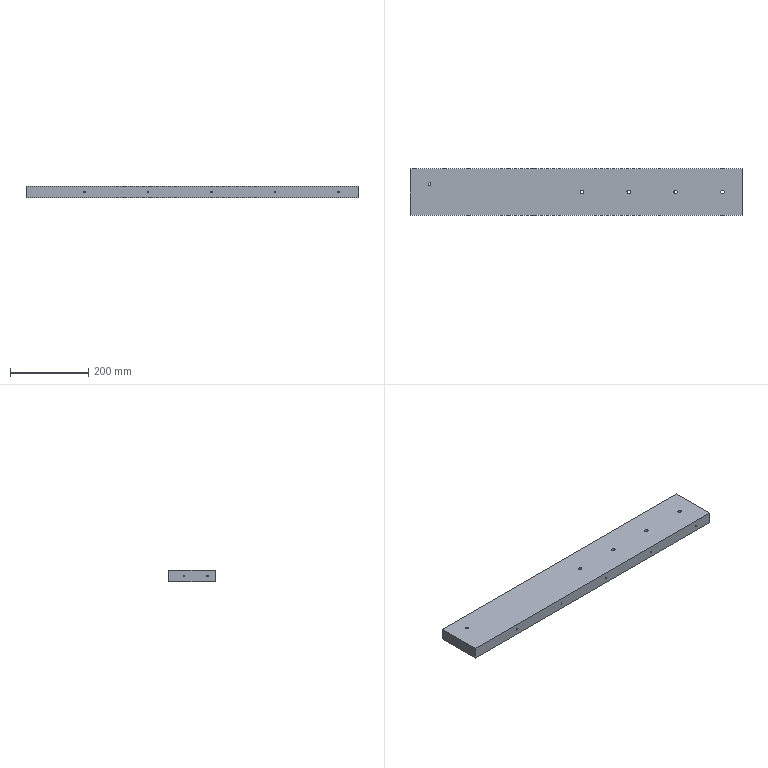Part | NX | 1 solid | 43 faces | box 850 x 120 x 30 mm | volume 3045845 mm3 | cylinder 21 | cone 16 | plane 6 | commonest cylinder face diameters 3.3 x12 9 x4 6.8 x3 8.5 x2
STEP:
#1=CARTESIAN_POINT('',(-425.,-60.,-15.));
#2=VERTEX_POINT('',#1);
#3=CARTESIAN_POINT('',(425.,-60.,-15.));
#4=VERTEX_POINT('',#3);
#5=CARTESIAN_POINT('',(-425.,-60.,-15.));
#6=DIRECTION('',(1.,0.,0.));
#7=VECTOR('',#6,1000.);
#8=LINE('',#5,#7);
#9=EDGE_CURVE('',#2,#4,#8,.T.);
#10=ORIENTED_EDGE('',*,*,#9,.T.);
#11=CARTESIAN_POINT('',(425.,-60.,15.));
#12=VERTEX_POINT('',#11);
#13=CARTESIAN_POINT('',(425.,-60.,15.));
#14=DIRECTION('',(0.,0.,-1.));
#15=VECTOR('',#14,1000.);
#16=LINE('',#13,#15);
#17=EDGE_CURVE('',#12,#4,#16,.T.);
#18=ORIENTED_EDGE('',*,*,#17,.F.);
#19=CARTESIAN_POINT('',(-425.,-60.,15.));
#20=VERTEX_POINT('',#19);
#21=CARTESIAN_POINT('',(-425.,-60.,15.));
#22=DIRECTION('',(1.,0.,0.));
#23=VECTOR('',#22,1000.);
#24=LINE('',#21,#23);
#25=EDGE_CURVE('',#20,#12,#24,.T.);
#26=ORIENTED_EDGE('',*,*,#25,.F.);
#27=CARTESIAN_POINT('',(-425.,-60.,15.));
#28=DIRECTION('',(0.,0.,-1.));
#29=VECTOR('',#28,1000.);
#30=LINE('',#27,#29);
#31=EDGE_CURVE('',#20,#2,#30,.T.);
#32=ORIENTED_EDGE('',*,*,#31,.T.);
#33=EDGE_LOOP('',(#10,#18,#26,#32));
#34=FACE_BOUND('',#33,.T.);
#35=CARTESIAN_POINT('',(375.,-60.,-1.65));
#36=VERTEX_POINT('',#35);
#37=CARTESIAN_POINT('',(375.,-60.,0.));
#38=DIRECTION('',(0.,-1.,0.));
#39=DIRECTION('',(0.,0.,-1.));
#40=AXIS2_PLACEMENT_3D('',#37,#38,#39);
#41=CIRCLE('',#40,1.65);
#42=EDGE_CURVE('',#36,#36,#41,.T.);
#43=ORIENTED_EDGE('',*,*,#42,.F.);
#44=EDGE_LOOP('',(#43));
#45=FACE_BOUND('',#44,.T.);
#46=CARTESIAN_POINT('',(212.5,-60.,-1.65));
#47=VERTEX_POINT('',#46);
#48=CARTESIAN_POINT('',(212.5,-60.,0.));
#49=DIRECTION('',(0.,-1.,0.));
#50=DIRECTION('',(0.,0.,-1.));
#51=AXIS2_PLACEMENT_3D('',#48,#49,#50);
#52=CIRCLE('',#51,1.65);
#53=EDGE_CURVE('',#47,#47,#52,.T.);
#54=ORIENTED_EDGE('',*,*,#53,.F.);
#55=EDGE_LOOP('',(#54));
#56=FACE_BOUND('',#55,.T.);
#57=CARTESIAN_POINT('',(50.,-60.,-1.65));
#58=VERTEX_POINT('',#57);
#59=CARTESIAN_POINT('',(50.,-60.,0.));
#60=DIRECTION('',(0.,-1.,0.));
#61=DIRECTION('',(0.,0.,-1.));
#62=AXIS2_PLACEMENT_3D('',#59,#60,#61);
#63=CIRCLE('',#62,1.65);
#64=EDGE_CURVE('',#58,#58,#63,.T.);
#65=ORIENTED_EDGE('',*,*,#64,.F.);
#66=EDGE_LOOP('',(#65));
#67=FACE_BOUND('',#66,.T.);
#68=CARTESIAN_POINT('',(-112.5,-60.,1.65));
#69=VERTEX_POINT('',#68);
#70=CARTESIAN_POINT('',(-112.5,-60.,0.));
#71=DIRECTION('',(0.,-1.,0.));
#72=DIRECTION('',(0.,0.,1.));
#73=AXIS2_PLACEMENT_3D('',#70,#71,#72);
#74=CIRCLE('',#73,1.65);
#75=EDGE_CURVE('',#69,#69,#74,.T.);
#76=ORIENTED_EDGE('',*,*,#75,.F.);
#77=EDGE_LOOP('',(#76));
#78=FACE_BOUND('',#77,.T.);
#79=CARTESIAN_POINT('',(-275.,-60.,1.65));
#80=VERTEX_POINT('',#79);
#81=CARTESIAN_POINT('',(-275.,-60.,0.));
#82=DIRECTION('',(0.,-1.,0.));
#83=DIRECTION('',(0.,0.,1.));
#84=AXIS2_PLACEMENT_3D('',#81,#82,#83);
#85=CIRCLE('',#84,1.65);
#86=EDGE_CURVE('',#80,#80,#85,.T.);
#87=ORIENTED_EDGE('',*,*,#86,.F.);
#88=EDGE_LOOP('',(#87));
#89=FACE_BOUND('',#88,.T.);
#90=CARTESIAN_POINT('',(-425.,-60.,15.));
#91=DIRECTION('',(0.,1.,0.));
#92=DIRECTION('',(0.,0.,1.));
#93=AXIS2_PLACEMENT_3D('',#90,#91,#92);
#94=PLANE('',#93);
#95=ADVANCED_FACE('',(#34,#45,#56,#67,#78,#89),#94,.F.);
#96=CARTESIAN_POINT('',(-425.,60.,-15.));
#97=VERTEX_POINT('',#96);
#98=CARTESIAN_POINT('',(-425.,-60.,-15.));
#99=DIRECTION('',(0.,1.,0.));
#100=VECTOR('',#99,1000.);
#101=LINE('',#98,#100);
#102=EDGE_CURVE('',#2,#97,#101,.T.);
#103=ORIENTED_EDGE('',*,*,#102,.F.);
#104=ORIENTED_EDGE('',*,*,#31,.F.);
#105=CARTESIAN_POINT('',(-425.,60.,15.));
#106=VERTEX_POINT('',#105);
#107=CARTESIAN_POINT('',(-425.,-60.,15.));
#108=DIRECTION('',(0.,1.,0.));
#109=VECTOR('',#108,1000.);
#110=LINE('',#107,#109);
#111=EDGE_CURVE('',#20,#106,#110,.T.);
#112=ORIENTED_EDGE('',*,*,#111,.T.);
#113=CARTESIAN_POINT('',(-425.,60.,15.));
#114=DIRECTION('',(0.,0.,-1.));
#115=VECTOR('',#114,1000.);
#116=LINE('',#113,#115);
#117=EDGE_CURVE('',#106,#97,#116,.T.);
#118=ORIENTED_EDGE('',*,*,#117,.T.);
#119=EDGE_LOOP('',(#103,#104,#112,#118));
#120=FACE_BOUND('',#119,.T.);
#121=CARTESIAN_POINT('',(-425.,20.,1.65));
#122=VERTEX_POINT('',#121);
#123=CARTESIAN_POINT('',(-425.,20.,0.));
#124=DIRECTION('',(-1.,0.,0.));
#125=DIRECTION('',(0.,0.,1.));
#126=AXIS2_PLACEMENT_3D('',#123,#124,#125);
#127=CIRCLE('',#126,1.65);
#128=EDGE_CURVE('',#122,#122,#127,.T.);
#129=ORIENTED_EDGE('',*,*,#128,.F.);
#130=EDGE_LOOP('',(#129));
#131=FACE_BOUND('',#130,.T.);
#132=CARTESIAN_POINT('',(-425.,-40.,1.65));
#133=VERTEX_POINT('',#132);
#134=CARTESIAN_POINT('',(-425.,-40.,0.));
#135=DIRECTION('',(-1.,0.,0.));
#136=DIRECTION('',(0.,0.,1.));
#137=AXIS2_PLACEMENT_3D('',#134,#135,#136);
#138=CIRCLE('',#137,1.65);
#139=EDGE_CURVE('',#133,#133,#138,.T.);
#140=ORIENTED_EDGE('',*,*,#139,.F.);
#141=EDGE_LOOP('',(#140));
#142=FACE_BOUND('',#141,.T.);
#143=CARTESIAN_POINT('',(-425.,-60.,15.));
#144=DIRECTION('',(-1.,0.,0.));
#145=DIRECTION('',(0.,0.,1.));
#146=AXIS2_PLACEMENT_3D('',#143,#144,#145);
#147=PLANE('',#146);
#148=ADVANCED_FACE('',(#120,#131,#142),#147,.T.);
#149=CARTESIAN_POINT('',(-335.,60.,3.4));
#150=VERTEX_POINT('',#149);
#151=CARTESIAN_POINT('',(-335.,60.,0.));
#152=DIRECTION('',(0.,1.,0.));
#153=DIRECTION('',(0.,0.,1.));
#154=AXIS2_PLACEMENT_3D('',#151,#152,#153);
#155=CIRCLE('',#154,3.4);
#156=EDGE_CURVE('',#150,#150,#155,.T.);
#157=ORIENTED_EDGE('',*,*,#156,.F.);
#158=EDGE_LOOP('',(#157));
#159=FACE_BOUND('',#158,.T.);
#160=CARTESIAN_POINT('',(425.,60.,15.));
#161=VERTEX_POINT('',#160);
#162=CARTESIAN_POINT('',(425.,60.,-15.));
#163=VERTEX_POINT('',#162);
#164=CARTESIAN_POINT('',(425.,60.,15.));
#165=DIRECTION('',(0.,0.,-1.));
#166=VECTOR('',#165,1000.);
#167=LINE('',#164,#166);
#168=EDGE_CURVE('',#161,#163,#167,.T.);
#169=ORIENTED_EDGE('',*,*,#168,.T.);
#170=CARTESIAN_POINT('',(-425.,60.,-15.));
#171=DIRECTION('',(1.,0.,0.));
#172=VECTOR('',#171,1000.);
#173=LINE('',#170,#172);
#174=EDGE_CURVE('',#163,#97,#173,.F.);
#175=ORIENTED_EDGE('',*,*,#174,.T.);
#176=ORIENTED_EDGE('',*,*,#117,.F.);
#177=CARTESIAN_POINT('',(-425.,60.,15.));
#178=DIRECTION('',(1.,0.,0.));
#179=VECTOR('',#178,1000.);
#180=LINE('',#177,#179);
#181=EDGE_CURVE('',#106,#161,#180,.T.);
#182=ORIENTED_EDGE('',*,*,#181,.T.);
#183=EDGE_LOOP('',(#169,#175,#176,#182));
#184=FACE_BOUND('',#183,.T.);
#185=CARTESIAN_POINT('',(-275.,60.,1.65));
#186=VERTEX_POINT('',#185);
#187=CARTESIAN_POINT('',(-275.,60.,0.));
#188=DIRECTION('',(0.,1.,0.));
#189=DIRECTION('',(0.,0.,1.));
#190=AXIS2_PLACEMENT_3D('',#187,#188,#189);
#191=CIRCLE('',#190,1.65);
#192=EDGE_CURVE('',#186,#186,#191,.T.);
#193=ORIENTED_EDGE('',*,*,#192,.F.);
#194=EDGE_LOOP('',(#193));
#195=FACE_BOUND('',#194,.T.);
#196=CARTESIAN_POINT('',(-112.5,60.,1.65));
#197=VERTEX_POINT('',#196);
#198=CARTESIAN_POINT('',(-112.5,60.,0.));
#199=DIRECTION('',(0.,1.,0.));
#200=DIRECTION('',(0.,0.,1.));
#201=AXIS2_PLACEMENT_3D('',#198,#199,#200);
#202=CIRCLE('',#201,1.65);
#203=EDGE_CURVE('',#197,#197,#202,.T.);
#204=ORIENTED_EDGE('',*,*,#203,.F.);
#205=EDGE_LOOP('',(#204));
#206=FACE_BOUND('',#205,.T.);
#207=CARTESIAN_POINT('',(50.,60.,1.65));
#208=VERTEX_POINT('',#207);
#209=CARTESIAN_POINT('',(50.,60.,0.));
#210=DIRECTION('',(0.,1.,0.));
#211=DIRECTION('',(0.,0.,1.));
#212=AXIS2_PLACEMENT_3D('',#209,#210,#211);
#213=CIRCLE('',#212,1.65);
#214=EDGE_CURVE('',#208,#208,#213,.T.);
#215=ORIENTED_EDGE('',*,*,#214,.F.);
#216=EDGE_LOOP('',(#215));
#217=FACE_BOUND('',#216,.T.);
#218=CARTESIAN_POINT('',(212.5,60.,1.65));
#219=VERTEX_POINT('',#218);
#220=CARTESIAN_POINT('',(212.5,60.,0.));
#221=DIRECTION('',(0.,1.,0.));
#222=DIRECTION('',(0.,0.,1.));
#223=AXIS2_PLACEMENT_3D('',#220,#221,#222);
#224=CIRCLE('',#223,1.65);
#225=EDGE_CURVE('',#219,#219,#224,.T.);
#226=ORIENTED_EDGE('',*,*,#225,.F.);
#227=EDGE_LOOP('',(#226));
#228=FACE_BOUND('',#227,.T.);
#229=CARTESIAN_POINT('',(375.,60.,1.65));
#230=VERTEX_POINT('',#229);
#231=CARTESIAN_POINT('',(375.,60.,0.));
#232=DIRECTION('',(0.,1.,0.));
#233=DIRECTION('',(0.,0.,1.));
#234=AXIS2_PLACEMENT_3D('',#231,#232,#233);
#235=CIRCLE('',#234,1.65);
#236=EDGE_CURVE('',#230,#230,#235,.T.);
#237=ORIENTED_EDGE('',*,*,#236,.F.);
#238=EDGE_LOOP('',(#237));
#239=FACE_BOUND('',#238,.T.);
#240=CARTESIAN_POINT('',(-415.,60.,3.4));
#241=VERTEX_POINT('',#240);
#242=CARTESIAN_POINT('',(-415.,60.,0.));
#243=DIRECTION('',(0.,1.,0.));
#244=DIRECTION('',(0.,0.,1.));
#245=AXIS2_PLACEMENT_3D('',#242,#243,#244);
#246=CIRCLE('',#245,3.4);
#247=EDGE_CURVE('',#241,#241,#246,.T.);
#248=ORIENTED_EDGE('',*,*,#247,.F.);
#249=EDGE_LOOP('',(#248));
#250=FACE_BOUND('',#249,.T.);
#251=CARTESIAN_POINT('',(-425.,60.,15.));
#252=DIRECTION('',(0.,1.,0.));
#253=DIRECTION('',(0.,0.,1.));
#254=AXIS2_PLACEMENT_3D('',#251,#252,#253);
#255=PLANE('',#254);
#256=ADVANCED_FACE('',(#159,#184,#195,#206,#217,#228,#239,#250),#255,.T.);
#257=ORIENTED_EDGE('',*,*,#168,.F.);
#258=CARTESIAN_POINT('',(425.,-60.,15.));
#259=DIRECTION('',(0.,-1.,0.));
#260=VECTOR('',#259,1000.);
#261=LINE('',#258,#260);
#262=EDGE_CURVE('',#161,#12,#261,.T.);
#263=ORIENTED_EDGE('',*,*,#262,.T.);
#264=ORIENTED_EDGE('',*,*,#17,.T.);
#265=CARTESIAN_POINT('',(425.,0.,-15.));
#266=DIRECTION('',(0.,1.,0.));
#267=VECTOR('',#266,1000.);
#268=LINE('',#265,#267);
#269=EDGE_CURVE('',#4,#163,#268,.T.);
#270=ORIENTED_EDGE('',*,*,#269,.T.);
#271=EDGE_LOOP('',(#257,#263,#264,#270));
#272=FACE_BOUND('',#271,.T.);
#273=CARTESIAN_POINT('',(425.,45.,-4.25));
#274=VERTEX_POINT('',#273);
#275=CARTESIAN_POINT('',(425.,45.,0.));
#276=DIRECTION('',(1.,0.,0.));
#277=DIRECTION('',(0.,0.,-1.));
#278=AXIS2_PLACEMENT_3D('',#275,#276,#277);
#279=CIRCLE('',#278,4.25);
#280=EDGE_CURVE('',#274,#274,#279,.T.);
#281=ORIENTED_EDGE('',*,*,#280,.F.);
#282=EDGE_LOOP('',(#281));
#283=FACE_BOUND('',#282,.T.);
#284=CARTESIAN_POINT('',(425.,-45.,-4.25));
#285=VERTEX_POINT('',#284);
#286=CARTESIAN_POINT('',(425.,-45.,0.));
#287=DIRECTION('',(1.,0.,0.));
#288=DIRECTION('',(0.,0.,-1.));
#289=AXIS2_PLACEMENT_3D('',#286,#287,#288);
#290=CIRCLE('',#289,4.25);
#291=EDGE_CURVE('',#285,#285,#290,.T.);
#292=ORIENTED_EDGE('',*,*,#291,.F.);
#293=EDGE_LOOP('',(#292));
#294=FACE_BOUND('',#293,.T.);
#295=CARTESIAN_POINT('',(425.,-60.,15.));
#296=DIRECTION('',(-1.,0.,0.));
#297=DIRECTION('',(0.,0.,1.));
#298=AXIS2_PLACEMENT_3D('',#295,#296,#297);
#299=PLANE('',#298);
#300=ADVANCED_FACE('',(#272,#283,#294),#299,.F.);
#301=CARTESIAN_POINT('',(139.5,0.,-15.));
#302=VERTEX_POINT('',#301);
#303=CARTESIAN_POINT('',(135.,0.,-15.));
#304=DIRECTION('',(0.,0.,1.));
#305=DIRECTION('',(1.,0.,0.));
#306=AXIS2_PLACEMENT_3D('',#303,#304,#305);
#307=CIRCLE('',#306,4.5);
#308=EDGE_CURVE('',#302,#302,#307,.T.);
#309=ORIENTED_EDGE('',*,*,#308,.T.);
#310=EDGE_LOOP('',(#309));
#311=FACE_BOUND('',#310,.T.);
#312=CARTESIAN_POINT('',(19.5,0.,-15.));
#313=VERTEX_POINT('',#312);
#314=CARTESIAN_POINT('',(15.,0.,-15.));
#315=DIRECTION('',(0.,0.,1.));
#316=DIRECTION('',(1.,0.,0.));
#317=AXIS2_PLACEMENT_3D('',#314,#315,#316);
#318=CIRCLE('',#317,4.5);
#319=EDGE_CURVE('',#313,#313,#318,.T.);
#320=ORIENTED_EDGE('',*,*,#319,.T.);
#321=EDGE_LOOP('',(#320));
#322=FACE_BOUND('',#321,.T.);
#323=ORIENTED_EDGE('',*,*,#174,.F.);
#324=ORIENTED_EDGE('',*,*,#269,.F.);
#325=ORIENTED_EDGE('',*,*,#9,.F.);
#326=ORIENTED_EDGE('',*,*,#102,.T.);
#327=EDGE_LOOP('',(#323,#324,#325,#326));
#328=FACE_BOUND('',#327,.T.);
#329=CARTESIAN_POINT('',(259.5,0.,-15.));
#330=VERTEX_POINT('',#329);
#331=CARTESIAN_POINT('',(255.,0.,-15.));
#332=DIRECTION('',(0.,0.,1.));
#333=DIRECTION('',(1.,0.,0.));
#334=AXIS2_PLACEMENT_3D('',#331,#332,#333);
#335=CIRCLE('',#334,4.5);
#336=EDGE_CURVE('',#330,#330,#335,.T.);
#337=ORIENTED_EDGE('',*,*,#336,.T.);
#338=EDGE_LOOP('',(#337));
#339=FACE_BOUND('',#338,.T.);
#340=CARTESIAN_POINT('',(379.5,0.,-15.));
#341=VERTEX_POINT('',#340);
#342=CARTESIAN_POINT('',(375.,0.,-15.));
#343=DIRECTION('',(0.,0.,1.));
#344=DIRECTION('',(1.,0.,0.));
#345=AXIS2_PLACEMENT_3D('',#342,#343,#344);
#346=CIRCLE('',#345,4.5);
#347=EDGE_CURVE('',#341,#341,#346,.T.);
#348=ORIENTED_EDGE('',*,*,#347,.T.);
#349=EDGE_LOOP('',(#348));
#350=FACE_BOUND('',#349,.T.);
#351=CARTESIAN_POINT('',(-378.4,20.,-15.));
#352=VERTEX_POINT('',#351);
#353=CARTESIAN_POINT('',(-375.,20.,-15.));
#354=DIRECTION('',(0.,0.,-1.));
#355=DIRECTION('',(-1.,0.,0.));
#356=AXIS2_PLACEMENT_3D('',#353,#354,#355);
#357=CIRCLE('',#356,3.4);
#358=EDGE_CURVE('',#352,#352,#357,.T.);
#359=ORIENTED_EDGE('',*,*,#358,.F.);
#360=EDGE_LOOP('',(#359));
#361=FACE_BOUND('',#360,.T.);
#362=CARTESIAN_POINT('',(0.,0.,-15.));
#363=DIRECTION('',(0.,0.,-1.));
#364=DIRECTION('',(-1.,0.,0.));
#365=AXIS2_PLACEMENT_3D('',#362,#363,#364);
#366=PLANE('',#365);
#367=ADVANCED_FACE('',(#311,#322,#328,#339,#350,#361),#366,.T.);
#368=CARTESIAN_POINT('',(259.5,0.,15.));
#369=VERTEX_POINT('',#368);
#370=CARTESIAN_POINT('',(255.,0.,15.));
#371=DIRECTION('',(0.,0.,1.));
#372=DIRECTION('',(1.,0.,0.));
#373=AXIS2_PLACEMENT_3D('',#370,#371,#372);
#374=CIRCLE('',#373,4.5);
#375=EDGE_CURVE('',#369,#369,#374,.T.);
#376=ORIENTED_EDGE('',*,*,#375,.F.);
#377=EDGE_LOOP('',(#376));
#378=FACE_BOUND('',#377,.T.);
#379=ORIENTED_EDGE('',*,*,#262,.F.);
#380=ORIENTED_EDGE('',*,*,#181,.F.);
#381=ORIENTED_EDGE('',*,*,#111,.F.);
#382=ORIENTED_EDGE('',*,*,#25,.T.);
#383=EDGE_LOOP('',(#379,#380,#381,#382));
#384=FACE_BOUND('',#383,.T.);
#385=CARTESIAN_POINT('',(19.5,0.,15.));
#386=VERTEX_POINT('',#385);
#387=CARTESIAN_POINT('',(15.,0.,15.));
#388=DIRECTION('',(0.,0.,1.));
#389=DIRECTION('',(1.,0.,0.));
#390=AXIS2_PLACEMENT_3D('',#387,#388,#389);
#391=CIRCLE('',#390,4.5);
#392=EDGE_CURVE('',#386,#386,#391,.T.);
#393=ORIENTED_EDGE('',*,*,#392,.F.);
#394=EDGE_LOOP('',(#393));
#395=FACE_BOUND('',#394,.T.);
#396=CARTESIAN_POINT('',(139.5,0.,15.));
#397=VERTEX_POINT('',#396);
#398=CARTESIAN_POINT('',(135.,0.,15.));
#399=DIRECTION('',(0.,0.,1.));
#400=DIRECTION('',(1.,0.,0.));
#401=AXIS2_PLACEMENT_3D('',#398,#399,#400);
#402=CIRCLE('',#401,4.5);
#403=EDGE_CURVE('',#397,#397,#402,.T.);
#404=ORIENTED_EDGE('',*,*,#403,.F.);
#405=EDGE_LOOP('',(#404));
#406=FACE_BOUND('',#405,.T.);
#407=CARTESIAN_POINT('',(379.5,0.,15.));
#408=VERTEX_POINT('',#407);
#409=CARTESIAN_POINT('',(375.,0.,15.));
#410=DIRECTION('',(0.,0.,1.));
#411=DIRECTION('',(1.,0.,0.));
#412=AXIS2_PLACEMENT_3D('',#409,#410,#411);
#413=CIRCLE('',#412,4.5);
#414=EDGE_CURVE('',#408,#408,#413,.T.);
#415=ORIENTED_EDGE('',*,*,#414,.F.);
#416=EDGE_LOOP('',(#415));
#417=FACE_BOUND('',#416,.T.);
#418=CARTESIAN_POINT('',(-378.4,20.,15.));
#419=VERTEX_POINT('',#418);
#420=CARTESIAN_POINT('',(-375.,20.,15.));
#421=DIRECTION('',(0.,0.,-1.));
#422=DIRECTION('',(-1.,0.,0.));
#423=AXIS2_PLACEMENT_3D('',#420,#421,#422);
#424=CIRCLE('',#423,3.4);
#425=EDGE_CURVE('',#419,#419,#424,.T.);
#426=ORIENTED_EDGE('',*,*,#425,.T.);
#427=EDGE_LOOP('',(#426));
#428=FACE_BOUND('',#427,.T.);
#429=CARTESIAN_POINT('',(0.,0.,15.));
#430=DIRECTION('',(0.,0.,-1.));
#431=DIRECTION('',(-1.,0.,0.));
#432=AXIS2_PLACEMENT_3D('',#429,#430,#431);
#433=PLANE('',#432);
#434=ADVANCED_FACE('',(#378,#384,#395,#406,#417,#428),#433,.F.);
#435=CARTESIAN_POINT('',(-335.,40.25,3.4));
#436=VERTEX_POINT('',#435);
#437=CARTESIAN_POINT('',(-335.,40.25,0.));
#438=DIRECTION('',(0.,1.,0.));
#439=DIRECTION('',(0.,0.,1.));
#440=AXIS2_PLACEMENT_3D('',#437,#438,#439);
#441=CIRCLE('',#440,3.4);
#442=EDGE_CURVE('',#436,#436,#441,.T.);
#443=ORIENTED_EDGE('',*,*,#442,.T.);
#444=EDGE_LOOP('',(#443));
#445=FACE_BOUND('',#444,.T.);
#446=CARTESIAN_POINT('',(-335.,38.207,0.));
#447=VERTEX_POINT('',#446);
#448=VERTEX_LOOP('',#447);
#449=FACE_BOUND('',#448,.T.);
#450=CARTESIAN_POINT('',(-335.,40.25,0.));
#451=DIRECTION('',(0.,1.,0.));
#452=DIRECTION('',(0.,0.,1.));
#453=AXIS2_PLACEMENT_3D('',#450,#451,#452);
#454=CONICAL_SURFACE('',#453,3.4,1.03);
#455=ADVANCED_FACE('',(#445,#449),#454,.F.);
#456=ORIENTED_EDGE('',*,*,#442,.F.);
#457=EDGE_LOOP('',(#456));
#458=FACE_BOUND('',#457,.T.);
#459=ORIENTED_EDGE('',*,*,#156,.T.);
#460=EDGE_LOOP('',(#459));
#461=FACE_BOUND('',#460,.T.);
#462=CARTESIAN_POINT('',(-335.,60.,0.));
#463=DIRECTION('',(0.,1.,0.));
#464=DIRECTION('',(0.,0.,1.));
#465=AXIS2_PLACEMENT_3D('',#462,#463,#464);
#466=CYLINDRICAL_SURFACE('',#465,3.4);
#467=ADVANCED_FACE('',(#458,#461),#466,.F.);
#468=CARTESIAN_POINT('',(-415.,40.25,3.4));
#469=VERTEX_POINT('',#468);
#470=CARTESIAN_POINT('',(-415.,40.25,0.));
#471=DIRECTION('',(0.,1.,0.));
#472=DIRECTION('',(0.,0.,1.));
#473=AXIS2_PLACEMENT_3D('',#470,#471,#472);
#474=CIRCLE('',#473,3.4);
#475=EDGE_CURVE('',#469,#469,#474,.T.);
#476=ORIENTED_EDGE('',*,*,#475,.T.);
#477=EDGE_LOOP('',(#476));
#478=FACE_BOUND('',#477,.T.);
#479=CARTESIAN_POINT('',(-415.,38.207,0.));
#480=VERTEX_POINT('',#479);
#481=VERTEX_LOOP('',#480);
#482=FACE_BOUND('',#481,.T.);
#483=CARTESIAN_POINT('',(-415.,40.25,0.));
#484=DIRECTION('',(0.,1.,0.));
#485=DIRECTION('',(0.,0.,1.));
#486=AXIS2_PLACEMENT_3D('',#483,#484,#485);
#487=CONICAL_SURFACE('',#486,3.4,1.03);
#488=ADVANCED_FACE('',(#478,#482),#487,.F.);
#489=ORIENTED_EDGE('',*,*,#475,.F.);
#490=EDGE_LOOP('',(#489));
#491=FACE_BOUND('',#490,.T.);
#492=ORIENTED_EDGE('',*,*,#247,.T.);
#493=EDGE_LOOP('',(#492));
#494=FACE_BOUND('',#493,.T.);
#495=CARTESIAN_POINT('',(-415.,60.,0.));
#496=DIRECTION('',(0.,1.,0.));
#497=DIRECTION('',(0.,0.,1.));
#498=AXIS2_PLACEMENT_3D('',#495,#496,#497);
#499=CYLINDRICAL_SURFACE('',#498,3.4);
#500=ADVANCED_FACE('',(#491,#494),#499,.F.);
#501=CARTESIAN_POINT('',(397.946,45.,0.));
#502=VERTEX_POINT('',#501);
#503=VERTEX_LOOP('',#502);
#504=FACE_BOUND('',#503,.T.);
#505=CARTESIAN_POINT('',(400.5,45.,-4.25));
#506=VERTEX_POINT('',#505);
#507=CARTESIAN_POINT('',(400.5,45.,0.));
#508=DIRECTION('',(1.,0.,0.));
#509=DIRECTION('',(0.,0.,-1.));
#510=AXIS2_PLACEMENT_3D('',#507,#508,#509);
#511=CIRCLE('',#510,4.25);
#512=EDGE_CURVE('',#506,#506,#511,.T.);
#513=ORIENTED_EDGE('',*,*,#512,.T.);
#514=EDGE_LOOP('',(#513));
#515=FACE_BOUND('',#514,.T.);
#516=CARTESIAN_POINT('',(400.5,45.,0.));
#517=DIRECTION('',(1.,0.,0.));
#518=DIRECTION('',(0.,0.,-1.));
#519=AXIS2_PLACEMENT_3D('',#516,#517,#518);
#520=CONICAL_SURFACE('',#519,4.25,1.03);
#521=ADVANCED_FACE('',(#504,#515),#520,.F.);
#522=ORIENTED_EDGE('',*,*,#280,.T.);
#523=EDGE_LOOP('',(#522));
#524=FACE_BOUND('',#523,.T.);
#525=ORIENTED_EDGE('',*,*,#512,.F.);
#526=EDGE_LOOP('',(#525));
#527=FACE_BOUND('',#526,.T.);
#528=CARTESIAN_POINT('',(425.,45.,0.));
#529=DIRECTION('',(1.,0.,0.));
#530=DIRECTION('',(0.,0.,-1.));
#531=AXIS2_PLACEMENT_3D('',#528,#529,#530);
#532=CYLINDRICAL_SURFACE('',#531,4.25);
#533=ADVANCED_FACE('',(#524,#527),#532,.F.);
#534=CARTESIAN_POINT('',(397.946,-45.,0.));
#535=VERTEX_POINT('',#534);
#536=VERTEX_LOOP('',#535);
#537=FACE_BOUND('',#536,.T.);
#538=CARTESIAN_POINT('',(400.5,-45.,-4.25));
#539=VERTEX_POINT('',#538);
#540=CARTESIAN_POINT('',(400.5,-45.,0.));
#541=DIRECTION('',(1.,0.,0.));
#542=DIRECTION('',(0.,0.,-1.));
#543=AXIS2_PLACEMENT_3D('',#540,#541,#542);
#544=CIRCLE('',#543,4.25);
#545=EDGE_CURVE('',#539,#539,#544,.T.);
#546=ORIENTED_EDGE('',*,*,#545,.T.);
#547=EDGE_LOOP('',(#546));
#548=FACE_BOUND('',#547,.T.);
#549=CARTESIAN_POINT('',(400.5,-45.,0.));
#550=DIRECTION('',(1.,0.,0.));
#551=DIRECTION('',(0.,0.,-1.));
#552=AXIS2_PLACEMENT_3D('',#549,#550,#551);
#553=CONICAL_SURFACE('',#552,4.25,1.03);
#554=ADVANCED_FACE('',(#537,#548),#553,.F.);
#555=ORIENTED_EDGE('',*,*,#291,.T.);
#556=EDGE_LOOP('',(#555));
#557=FACE_BOUND('',#556,.T.);
#558=ORIENTED_EDGE('',*,*,#545,.F.);
#559=EDGE_LOOP('',(#558));
#560=FACE_BOUND('',#559,.T.);
#561=CARTESIAN_POINT('',(425.,-45.,0.));
#562=DIRECTION('',(1.,0.,0.));
#563=DIRECTION('',(0.,0.,-1.));
#564=AXIS2_PLACEMENT_3D('',#561,#562,#563);
#565=CYLINDRICAL_SURFACE('',#564,4.25);
#566=ADVANCED_FACE('',(#557,#560),#565,.F.);
#567=ORIENTED_EDGE('',*,*,#319,.F.);
#568=EDGE_LOOP('',(#567));
#569=FACE_BOUND('',#568,.T.);
#570=ORIENTED_EDGE('',*,*,#392,.T.);
#571=EDGE_LOOP('',(#570));
#572=FACE_BOUND('',#571,.T.);
#573=CARTESIAN_POINT('',(15.,0.,15.));
#574=DIRECTION('',(0.,0.,1.));
#575=DIRECTION('',(1.,0.,0.));
#576=AXIS2_PLACEMENT_3D('',#573,#574,#575);
#577=CYLINDRICAL_SURFACE('',#576,4.5);
#578=ADVANCED_FACE('',(#569,#572),#577,.F.);
#579=ORIENTED_EDGE('',*,*,#308,.F.);
#580=EDGE_LOOP('',(#579));
#581=FACE_BOUND('',#580,.T.);
#582=ORIENTED_EDGE('',*,*,#403,.T.);
#583=EDGE_LOOP('',(#582));
#584=FACE_BOUND('',#583,.T.);
#585=CARTESIAN_POINT('',(135.,0.,15.));
#586=DIRECTION('',(0.,0.,1.));
#587=DIRECTION('',(1.,0.,0.));
#588=AXIS2_PLACEMENT_3D('',#585,#586,#587);
#589=CYLINDRICAL_SURFACE('',#588,4.5);
#590=ADVANCED_FACE('',(#581,#584),#589,.F.);
#591=ORIENTED_EDGE('',*,*,#336,.F.);
#592=EDGE_LOOP('',(#591));
#593=FACE_BOUND('',#592,.T.);
#594=ORIENTED_EDGE('',*,*,#375,.T.);
#595=EDGE_LOOP('',(#594));
#596=FACE_BOUND('',#595,.T.);
#597=CARTESIAN_POINT('',(255.,0.,15.));
#598=DIRECTION('',(0.,0.,1.));
#599=DIRECTION('',(1.,0.,0.));
#600=AXIS2_PLACEMENT_3D('',#597,#598,#599);
#601=CYLINDRICAL_SURFACE('',#600,4.5);
#602=ADVANCED_FACE('',(#593,#596),#601,.F.);
#603=ORIENTED_EDGE('',*,*,#347,.F.);
#604=EDGE_LOOP('',(#603));
#605=FACE_BOUND('',#604,.T.);
#606=ORIENTED_EDGE('',*,*,#414,.T.);
#607=EDGE_LOOP('',(#606));
#608=FACE_BOUND('',#607,.T.);
#609=CARTESIAN_POINT('',(375.,0.,15.));
#610=DIRECTION('',(0.,0.,1.));
#611=DIRECTION('',(1.,0.,0.));
#612=AXIS2_PLACEMENT_3D('',#609,#610,#611);
#613=CYLINDRICAL_SURFACE('',#612,4.5);
#614=ADVANCED_FACE('',(#605,#608),#613,.F.);
#615=ORIENTED_EDGE('',*,*,#358,.T.);
#616=EDGE_LOOP('',(#615));
#617=FACE_BOUND('',#616,.T.);
#618=ORIENTED_EDGE('',*,*,#425,.F.);
#619=EDGE_LOOP('',(#618));
#620=FACE_BOUND('',#619,.T.);
#621=CARTESIAN_POINT('',(-375.,20.,-15.));
#622=DIRECTION('',(0.,0.,-1.));
#623=DIRECTION('',(-1.,0.,0.));
#624=AXIS2_PLACEMENT_3D('',#621,#622,#623);
#625=CYLINDRICAL_SURFACE('',#624,3.4);
#626=ADVANCED_FACE('',(#617,#620),#625,.F.);
#627=CARTESIAN_POINT('',(-275.,49.9,1.65));
#628=VERTEX_POINT('',#627);
#629=CARTESIAN_POINT('',(-275.,49.9,0.));
#630=DIRECTION('',(0.,1.,0.));
#631=DIRECTION('',(0.,0.,1.));
#632=AXIS2_PLACEMENT_3D('',#629,#630,#631);
#633=CIRCLE('',#632,1.65);
#634=EDGE_CURVE('',#628,#628,#633,.T.);
#635=ORIENTED_EDGE('',*,*,#634,.T.);
#636=EDGE_LOOP('',(#635));
#637=FACE_BOUND('',#636,.T.);
#638=CARTESIAN_POINT('',(-275.,48.909,0.));
#639=VERTEX_POINT('',#638);
#640=VERTEX_LOOP('',#639);
#641=FACE_BOUND('',#640,.T.);
#642=CARTESIAN_POINT('',(-275.,49.9,0.));
#643=DIRECTION('',(0.,1.,0.));
#644=DIRECTION('',(0.,0.,1.));
#645=AXIS2_PLACEMENT_3D('',#642,#643,#644);
#646=CONICAL_SURFACE('',#645,1.65,1.03);
#647=ADVANCED_FACE('',(#637,#641),#646,.F.);
#648=ORIENTED_EDGE('',*,*,#634,.F.);
#649=EDGE_LOOP('',(#648));
#650=FACE_BOUND('',#649,.T.);
#651=ORIENTED_EDGE('',*,*,#192,.T.);
#652=EDGE_LOOP('',(#651));
#653=FACE_BOUND('',#652,.T.);
#654=CARTESIAN_POINT('',(-275.,60.,0.));
#655=DIRECTION('',(0.,1.,0.));
#656=DIRECTION('',(0.,0.,1.));
#657=AXIS2_PLACEMENT_3D('',#654,#655,#656);
#658=CYLINDRICAL_SURFACE('',#657,1.65);
#659=ADVANCED_FACE('',(#650,#653),#658,.F.);
#660=CARTESIAN_POINT('',(-112.5,49.9,1.65));
#661=VERTEX_POINT('',#660);
#662=CARTESIAN_POINT('',(-112.5,49.9,0.));
#663=DIRECTION('',(0.,1.,0.));
#664=DIRECTION('',(0.,0.,1.));
#665=AXIS2_PLACEMENT_3D('',#662,#663,#664);
#666=CIRCLE('',#665,1.65);
#667=EDGE_CURVE('',#661,#661,#666,.T.);
#668=ORIENTED_EDGE('',*,*,#667,.T.);
#669=EDGE_LOOP('',(#668));
#670=FACE_BOUND('',#669,.T.);
#671=CARTESIAN_POINT('',(-112.5,48.909,0.));
#672=VERTEX_POINT('',#671);
#673=VERTEX_LOOP('',#672);
#674=FACE_BOUND('',#673,.T.);
#675=CARTESIAN_POINT('',(-112.5,49.9,0.));
#676=DIRECTION('',(0.,1.,0.));
#677=DIRECTION('',(0.,0.,1.));
#678=AXIS2_PLACEMENT_3D('',#675,#676,#677);
#679=CONICAL_SURFACE('',#678,1.65,1.03);
#680=ADVANCED_FACE('',(#670,#674),#679,.F.);
#681=ORIENTED_EDGE('',*,*,#667,.F.);
#682=EDGE_LOOP('',(#681));
#683=FACE_BOUND('',#682,.T.);
#684=ORIENTED_EDGE('',*,*,#203,.T.);
#685=EDGE_LOOP('',(#684));
#686=FACE_BOUND('',#685,.T.);
#687=CARTESIAN_POINT('',(-112.5,60.,0.));
#688=DIRECTION('',(0.,1.,0.));
#689=DIRECTION('',(0.,0.,1.));
#690=AXIS2_PLACEMENT_3D('',#687,#688,#689);
#691=CYLINDRICAL_SURFACE('',#690,1.65);
#692=ADVANCED_FACE('',(#683,#686),#691,.F.);
#693=CARTESIAN_POINT('',(50.,49.9,1.65));
#694=VERTEX_POINT('',#693);
#695=CARTESIAN_POINT('',(50.,49.9,0.));
#696=DIRECTION('',(0.,1.,0.));
#697=DIRECTION('',(0.,0.,1.));
#698=AXIS2_PLACEMENT_3D('',#695,#696,#697);
#699=CIRCLE('',#698,1.65);
#700=EDGE_CURVE('',#694,#694,#699,.T.);
#701=ORIENTED_EDGE('',*,*,#700,.T.);
#702=EDGE_LOOP('',(#701));
#703=FACE_BOUND('',#702,.T.);
#704=CARTESIAN_POINT('',(50.,48.909,0.));
#705=VERTEX_POINT('',#704);
#706=VERTEX_LOOP('',#705);
#707=FACE_BOUND('',#706,.T.);
#708=CARTESIAN_POINT('',(50.,49.9,0.));
#709=DIRECTION('',(0.,1.,0.));
#710=DIRECTION('',(0.,0.,1.));
#711=AXIS2_PLACEMENT_3D('',#708,#709,#710);
#712=CONICAL_SURFACE('',#711,1.65,1.03);
#713=ADVANCED_FACE('',(#703,#707),#712,.F.);
#714=ORIENTED_EDGE('',*,*,#700,.F.);
#715=EDGE_LOOP('',(#714));
#716=FACE_BOUND('',#715,.T.);
#717=ORIENTED_EDGE('',*,*,#214,.T.);
#718=EDGE_LOOP('',(#717));
#719=FACE_BOUND('',#718,.T.);
#720=CARTESIAN_POINT('',(50.,-60.,0.));
#721=DIRECTION('',(0.,-1.,0.));
#722=DIRECTION('',(0.,0.,-1.));
#723=AXIS2_PLACEMENT_3D('',#720,#721,#722);
#724=CYLINDRICAL_SURFACE('',#723,1.65);
#725=ADVANCED_FACE('',(#716,#719),#724,.F.);
#726=CARTESIAN_POINT('',(212.5,49.9,1.65));
#727=VERTEX_POINT('',#726);
#728=CARTESIAN_POINT('',(212.5,49.9,0.));
#729=DIRECTION('',(0.,1.,0.));
#730=DIRECTION('',(0.,0.,1.));
#731=AXIS2_PLACEMENT_3D('',#728,#729,#730);
#732=CIRCLE('',#731,1.65);
#733=EDGE_CURVE('',#727,#727,#732,.T.);
#734=ORIENTED_EDGE('',*,*,#733,.T.);
#735=EDGE_LOOP('',(#734));
#736=FACE_BOUND('',#735,.T.);
#737=CARTESIAN_POINT('',(212.5,48.909,0.));
#738=VERTEX_POINT('',#737);
#739=VERTEX_LOOP('',#738);
#740=FACE_BOUND('',#739,.T.);
#741=CARTESIAN_POINT('',(212.5,49.9,0.));
#742=DIRECTION('',(0.,1.,0.));
#743=DIRECTION('',(0.,0.,1.));
#744=AXIS2_PLACEMENT_3D('',#741,#742,#743);
#745=CONICAL_SURFACE('',#744,1.65,1.03);
#746=ADVANCED_FACE('',(#736,#740),#745,.F.);
#747=ORIENTED_EDGE('',*,*,#733,.F.);
#748=EDGE_LOOP('',(#747));
#749=FACE_BOUND('',#748,.T.);
#750=ORIENTED_EDGE('',*,*,#225,.T.);
#751=EDGE_LOOP('',(#750));
#752=FACE_BOUND('',#751,.T.);
#753=CARTESIAN_POINT('',(212.5,-60.,0.));
#754=DIRECTION('',(0.,-1.,0.));
#755=DIRECTION('',(0.,0.,-1.));
#756=AXIS2_PLACEMENT_3D('',#753,#754,#755);
#757=CYLINDRICAL_SURFACE('',#756,1.65);
#758=ADVANCED_FACE('',(#749,#752),#757,.F.);
#759=CARTESIAN_POINT('',(375.,49.9,1.65));
#760=VERTEX_POINT('',#759);
#761=CARTESIAN_POINT('',(375.,49.9,0.));
#762=DIRECTION('',(0.,1.,0.));
#763=DIRECTION('',(0.,0.,1.));
#764=AXIS2_PLACEMENT_3D('',#761,#762,#763);
#765=CIRCLE('',#764,1.65);
#766=EDGE_CURVE('',#760,#760,#765,.T.);
#767=ORIENTED_EDGE('',*,*,#766,.T.);
#768=EDGE_LOOP('',(#767));
#769=FACE_BOUND('',#768,.T.);
#770=CARTESIAN_POINT('',(375.,48.909,0.));
#771=VERTEX_POINT('',#770);
#772=VERTEX_LOOP('',#771);
#773=FACE_BOUND('',#772,.T.);
#774=CARTESIAN_POINT('',(375.,49.9,0.));
#775=DIRECTION('',(0.,1.,0.));
#776=DIRECTION('',(0.,0.,1.));
#777=AXIS2_PLACEMENT_3D('',#774,#775,#776);
#778=CONICAL_SURFACE('',#777,1.65,1.03);
#779=ADVANCED_FACE('',(#769,#773),#778,.F.);
#780=ORIENTED_EDGE('',*,*,#766,.F.);
#781=EDGE_LOOP('',(#780));
#782=FACE_BOUND('',#781,.T.);
#783=ORIENTED_EDGE('',*,*,#236,.T.);
#784=EDGE_LOOP('',(#783));
#785=FACE_BOUND('',#784,.T.);
#786=CARTESIAN_POINT('',(375.,-60.,0.));
#787=DIRECTION('',(0.,-1.,0.));
#788=DIRECTION('',(0.,0.,-1.));
#789=AXIS2_PLACEMENT_3D('',#786,#787,#788);
#790=CYLINDRICAL_SURFACE('',#789,1.65);
#791=ADVANCED_FACE('',(#782,#785),#790,.F.);
#792=CARTESIAN_POINT('',(375.,-48.909,0.));
#793=VERTEX_POINT('',#792);
#794=VERTEX_LOOP('',#793);
#795=FACE_BOUND('',#794,.T.);
#796=CARTESIAN_POINT('',(375.,-49.9,-1.65));
#797=VERTEX_POINT('',#796);
#798=CARTESIAN_POINT('',(375.,-49.9,0.));
#799=DIRECTION('',(0.,-1.,0.));
#800=DIRECTION('',(0.,0.,-1.));
#801=AXIS2_PLACEMENT_3D('',#798,#799,#800);
#802=CIRCLE('',#801,1.65);
#803=EDGE_CURVE('',#797,#797,#802,.T.);
#804=ORIENTED_EDGE('',*,*,#803,.T.);
#805=EDGE_LOOP('',(#804));
#806=FACE_BOUND('',#805,.T.);
#807=CARTESIAN_POINT('',(375.,-49.9,0.));
#808=DIRECTION('',(0.,-1.,0.));
#809=DIRECTION('',(0.,0.,-1.));
#810=AXIS2_PLACEMENT_3D('',#807,#808,#809);
#811=CONICAL_SURFACE('',#810,1.65,1.03);
#812=ADVANCED_FACE('',(#795,#806),#811,.F.);
#813=ORIENTED_EDGE('',*,*,#42,.T.);
#814=EDGE_LOOP('',(#813));
#815=FACE_BOUND('',#814,.T.);
#816=ORIENTED_EDGE('',*,*,#803,.F.);
#817=EDGE_LOOP('',(#816));
#818=FACE_BOUND('',#817,.T.);
#819=CARTESIAN_POINT('',(375.,-60.,0.));
#820=DIRECTION('',(0.,-1.,0.));
#821=DIRECTION('',(0.,0.,-1.));
#822=AXIS2_PLACEMENT_3D('',#819,#820,#821);
#823=CYLINDRICAL_SURFACE('',#822,1.65);
#824=ADVANCED_FACE('',(#815,#818),#823,.F.);
#825=CARTESIAN_POINT('',(212.5,-48.909,0.));
#826=VERTEX_POINT('',#825);
#827=VERTEX_LOOP('',#826);
#828=FACE_BOUND('',#827,.T.);
#829=CARTESIAN_POINT('',(212.5,-49.9,-1.65));
#830=VERTEX_POINT('',#829);
#831=CARTESIAN_POINT('',(212.5,-49.9,0.));
#832=DIRECTION('',(0.,-1.,0.));
#833=DIRECTION('',(0.,0.,-1.));
#834=AXIS2_PLACEMENT_3D('',#831,#832,#833);
#835=CIRCLE('',#834,1.65);
#836=EDGE_CURVE('',#830,#830,#835,.T.);
#837=ORIENTED_EDGE('',*,*,#836,.T.);
#838=EDGE_LOOP('',(#837));
#839=FACE_BOUND('',#838,.T.);
#840=CARTESIAN_POINT('',(212.5,-49.9,0.));
#841=DIRECTION('',(0.,-1.,0.));
#842=DIRECTION('',(0.,0.,-1.));
#843=AXIS2_PLACEMENT_3D('',#840,#841,#842);
#844=CONICAL_SURFACE('',#843,1.65,1.03);
#845=ADVANCED_FACE('',(#828,#839),#844,.F.);
#846=ORIENTED_EDGE('',*,*,#53,.T.);
#847=EDGE_LOOP('',(#846));
#848=FACE_BOUND('',#847,.T.);
#849=ORIENTED_EDGE('',*,*,#836,.F.);
#850=EDGE_LOOP('',(#849));
#851=FACE_BOUND('',#850,.T.);
#852=CARTESIAN_POINT('',(212.5,-60.,0.));
#853=DIRECTION('',(0.,-1.,0.));
#854=DIRECTION('',(0.,0.,-1.));
#855=AXIS2_PLACEMENT_3D('',#852,#853,#854);
#856=CYLINDRICAL_SURFACE('',#855,1.65);
#857=ADVANCED_FACE('',(#848,#851),#856,.F.);
#858=CARTESIAN_POINT('',(50.,-48.909,0.));
#859=VERTEX_POINT('',#858);
#860=VERTEX_LOOP('',#859);
#861=FACE_BOUND('',#860,.T.);
#862=CARTESIAN_POINT('',(50.,-49.9,-1.65));
#863=VERTEX_POINT('',#862);
#864=CARTESIAN_POINT('',(50.,-49.9,0.));
#865=DIRECTION('',(0.,-1.,0.));
#866=DIRECTION('',(0.,0.,-1.));
#867=AXIS2_PLACEMENT_3D('',#864,#865,#866);
#868=CIRCLE('',#867,1.65);
#869=EDGE_CURVE('',#863,#863,#868,.T.);
#870=ORIENTED_EDGE('',*,*,#869,.T.);
#871=EDGE_LOOP('',(#870));
#872=FACE_BOUND('',#871,.T.);
#873=CARTESIAN_POINT('',(50.,-49.9,0.));
#874=DIRECTION('',(0.,-1.,0.));
#875=DIRECTION('',(0.,0.,-1.));
#876=AXIS2_PLACEMENT_3D('',#873,#874,#875);
#877=CONICAL_SURFACE('',#876,1.65,1.03);
#878=ADVANCED_FACE('',(#861,#872),#877,.F.);
#879=ORIENTED_EDGE('',*,*,#64,.T.);
#880=EDGE_LOOP('',(#879));
#881=FACE_BOUND('',#880,.T.);
#882=ORIENTED_EDGE('',*,*,#869,.F.);
#883=EDGE_LOOP('',(#882));
#884=FACE_BOUND('',#883,.T.);
#885=CARTESIAN_POINT('',(50.,-60.,0.));
#886=DIRECTION('',(0.,-1.,0.));
#887=DIRECTION('',(0.,0.,-1.));
#888=AXIS2_PLACEMENT_3D('',#885,#886,#887);
#889=CYLINDRICAL_SURFACE('',#888,1.65);
#890=ADVANCED_FACE('',(#881,#884),#889,.F.);
#891=CARTESIAN_POINT('',(-112.5,-48.909,0.));
#892=VERTEX_POINT('',#891);
#893=VERTEX_LOOP('',#892);
#894=FACE_BOUND('',#893,.T.);
#895=CARTESIAN_POINT('',(-112.5,-49.9,-1.65));
#896=VERTEX_POINT('',#895);
#897=CARTESIAN_POINT('',(-112.5,-49.9,0.));
#898=DIRECTION('',(0.,-1.,0.));
#899=DIRECTION('',(0.,0.,-1.));
#900=AXIS2_PLACEMENT_3D('',#897,#898,#899);
#901=CIRCLE('',#900,1.65);
#902=EDGE_CURVE('',#896,#896,#901,.T.);
#903=ORIENTED_EDGE('',*,*,#902,.T.);
#904=EDGE_LOOP('',(#903));
#905=FACE_BOUND('',#904,.T.);
#906=CARTESIAN_POINT('',(-112.5,-49.9,0.));
#907=DIRECTION('',(0.,-1.,0.));
#908=DIRECTION('',(0.,0.,-1.));
#909=AXIS2_PLACEMENT_3D('',#906,#907,#908);
#910=CONICAL_SURFACE('',#909,1.65,1.03);
#911=ADVANCED_FACE('',(#894,#905),#910,.F.);
#912=ORIENTED_EDGE('',*,*,#75,.T.);
#913=EDGE_LOOP('',(#912));
#914=FACE_BOUND('',#913,.T.);
#915=ORIENTED_EDGE('',*,*,#902,.F.);
#916=EDGE_LOOP('',(#915));
#917=FACE_BOUND('',#916,.T.);
#918=CARTESIAN_POINT('',(-112.5,60.,0.));
#919=DIRECTION('',(0.,1.,0.));
#920=DIRECTION('',(0.,0.,1.));
#921=AXIS2_PLACEMENT_3D('',#918,#919,#920);
#922=CYLINDRICAL_SURFACE('',#921,1.65);
#923=ADVANCED_FACE('',(#914,#917),#922,.F.);
#924=CARTESIAN_POINT('',(-275.,-48.909,0.));
#925=VERTEX_POINT('',#924);
#926=VERTEX_LOOP('',#925);
#927=FACE_BOUND('',#926,.T.);
#928=CARTESIAN_POINT('',(-275.,-49.9,-1.65));
#929=VERTEX_POINT('',#928);
#930=CARTESIAN_POINT('',(-275.,-49.9,0.));
#931=DIRECTION('',(0.,-1.,0.));
#932=DIRECTION('',(0.,0.,-1.));
#933=AXIS2_PLACEMENT_3D('',#930,#931,#932);
#934=CIRCLE('',#933,1.65);
#935=EDGE_CURVE('',#929,#929,#934,.T.);
#936=ORIENTED_EDGE('',*,*,#935,.T.);
#937=EDGE_LOOP('',(#936));
#938=FACE_BOUND('',#937,.T.);
#939=CARTESIAN_POINT('',(-275.,-49.9,0.));
#940=DIRECTION('',(0.,-1.,0.));
#941=DIRECTION('',(0.,0.,-1.));
#942=AXIS2_PLACEMENT_3D('',#939,#940,#941);
#943=CONICAL_SURFACE('',#942,1.65,1.03);
#944=ADVANCED_FACE('',(#927,#938),#943,.F.);
#945=ORIENTED_EDGE('',*,*,#86,.T.);
#946=EDGE_LOOP('',(#945));
#947=FACE_BOUND('',#946,.T.);
#948=ORIENTED_EDGE('',*,*,#935,.F.);
#949=EDGE_LOOP('',(#948));
#950=FACE_BOUND('',#949,.T.);
#951=CARTESIAN_POINT('',(-275.,60.,0.));
#952=DIRECTION('',(0.,1.,0.));
#953=DIRECTION('',(0.,0.,1.));
#954=AXIS2_PLACEMENT_3D('',#951,#952,#953);
#955=CYLINDRICAL_SURFACE('',#954,1.65);
#956=ADVANCED_FACE('',(#947,#950),#955,.F.);
#957=CARTESIAN_POINT('',(-414.9,20.,1.65));
#958=VERTEX_POINT('',#957);
#959=CARTESIAN_POINT('',(-414.9,20.,0.));
#960=DIRECTION('',(-1.,0.,0.));
#961=DIRECTION('',(0.,0.,1.));
#962=AXIS2_PLACEMENT_3D('',#959,#960,#961);
#963=CIRCLE('',#962,1.65);
#964=EDGE_CURVE('',#958,#958,#963,.T.);
#965=ORIENTED_EDGE('',*,*,#964,.T.);
#966=EDGE_LOOP('',(#965));
#967=FACE_BOUND('',#966,.T.);
#968=CARTESIAN_POINT('',(-413.909,20.,0.));
#969=VERTEX_POINT('',#968);
#970=VERTEX_LOOP('',#969);
#971=FACE_BOUND('',#970,.T.);
#972=CARTESIAN_POINT('',(-414.9,20.,0.));
#973=DIRECTION('',(-1.,0.,0.));
#974=DIRECTION('',(0.,0.,1.));
#975=AXIS2_PLACEMENT_3D('',#972,#973,#974);
#976=CONICAL_SURFACE('',#975,1.65,1.03);
#977=ADVANCED_FACE('',(#967,#971),#976,.F.);
#978=ORIENTED_EDGE('',*,*,#964,.F.);
#979=EDGE_LOOP('',(#978));
#980=FACE_BOUND('',#979,.T.);
#981=ORIENTED_EDGE('',*,*,#128,.T.);
#982=EDGE_LOOP('',(#981));
#983=FACE_BOUND('',#982,.T.);
#984=CARTESIAN_POINT('',(-425.,20.,0.));
#985=DIRECTION('',(-1.,0.,0.));
#986=DIRECTION('',(0.,0.,1.));
#987=AXIS2_PLACEMENT_3D('',#984,#985,#986);
#988=CYLINDRICAL_SURFACE('',#987,1.65);
#989=ADVANCED_FACE('',(#980,#983),#988,.F.);
#990=CARTESIAN_POINT('',(-414.9,-40.,1.65));
#991=VERTEX_POINT('',#990);
#992=CARTESIAN_POINT('',(-414.9,-40.,0.));
#993=DIRECTION('',(-1.,0.,0.));
#994=DIRECTION('',(0.,0.,1.));
#995=AXIS2_PLACEMENT_3D('',#992,#993,#994);
#996=CIRCLE('',#995,1.65);
#997=EDGE_CURVE('',#991,#991,#996,.T.);
#998=ORIENTED_EDGE('',*,*,#997,.T.);
#999=EDGE_LOOP('',(#998));
#1000=FACE_BOUND('',#999,.T.);
#1001=CARTESIAN_POINT('',(-413.909,-40.,0.));
#1002=VERTEX_POINT('',#1001);
#1003=VERTEX_LOOP('',#1002);
#1004=FACE_BOUND('',#1003,.T.);
#1005=CARTESIAN_POINT('',(-414.9,-40.,0.));
#1006=DIRECTION('',(-1.,0.,0.));
#1007=DIRECTION('',(0.,0.,1.));
#1008=AXIS2_PLACEMENT_3D('',#1005,#1006,#1007);
#1009=CONICAL_SURFACE('',#1008,1.65,1.03);
#1010=ADVANCED_FACE('',(#1000,#1004),#1009,.F.);
#1011=ORIENTED_EDGE('',*,*,#997,.F.);
#1012=EDGE_LOOP('',(#1011));
#1013=FACE_BOUND('',#1012,.T.);
#1014=ORIENTED_EDGE('',*,*,#139,.T.);
#1015=EDGE_LOOP('',(#1014));
#1016=FACE_BOUND('',#1015,.T.);
#1017=CARTESIAN_POINT('',(-425.,-40.,0.));
#1018=DIRECTION('',(-1.,0.,0.));
#1019=DIRECTION('',(0.,0.,1.));
#1020=AXIS2_PLACEMENT_3D('',#1017,#1018,#1019);
#1021=CYLINDRICAL_SURFACE('',#1020,1.65);
#1022=ADVANCED_FACE('',(#1013,#1016),#1021,.F.);
#1023=CLOSED_SHELL('',(#95,#148,#256,#300,#367,#434,#455,#467,#488,#500,#521,#533,#554,#566,#578,#590,#602,#614,#626,#647,#659,#680,#692,#713,#725,#746,#758,#779,#791,#812,#824,#845,#857,#878,#890,#911,#923,#944,#956,#977,#989,#1010,#1022));
#1024=MANIFOLD_SOLID_BREP('',#1023);
#1025=(LENGTH_UNIT()NAMED_UNIT(*)SI_UNIT(.MILLI.,.METRE.));
#1026=UNCERTAINTY_MEASURE_WITH_UNIT(LENGTH_MEASURE(0.00001),#1025,'','');
#1027=(NAMED_UNIT(*)PLANE_ANGLE_UNIT()SI_UNIT($,.RADIAN.));
#1028=(NAMED_UNIT(*)SI_UNIT($,.STERADIAN.)SOLID_ANGLE_UNIT());
#1029=(GEOMETRIC_REPRESENTATION_CONTEXT(3)GLOBAL_UNCERTAINTY_ASSIGNED_CONTEXT((#1026))GLOBAL_UNIT_ASSIGNED_CONTEXT((#1025,#1027,#1028))REPRESENTATION_CONTEXT('',''));
#1030=ADVANCED_BREP_SHAPE_REPRESENTATION('',(#1024),#1029);